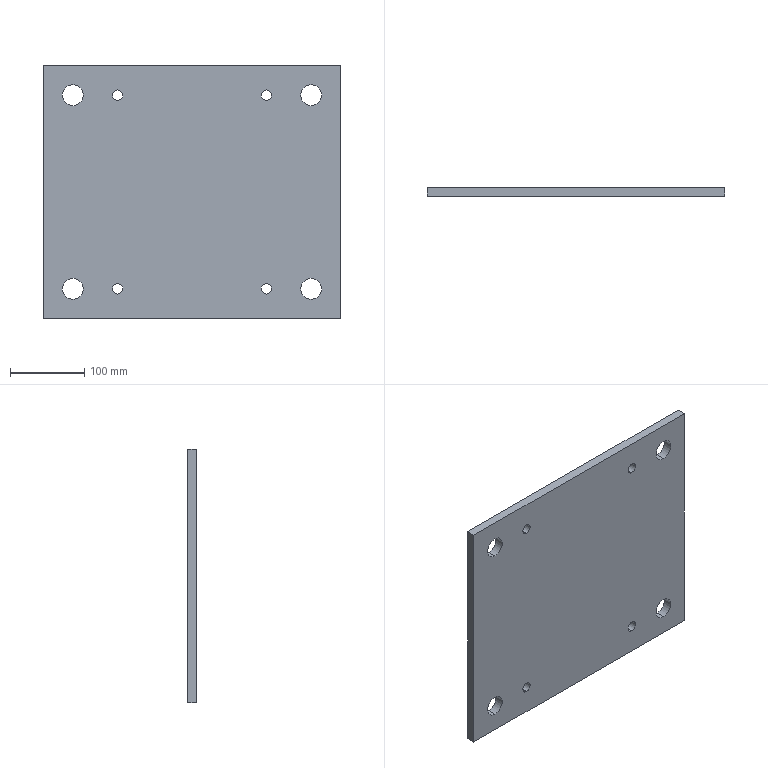Part | STEP file | Column base plate-Transfer kettle | 1 solid | 22 faces | box 400 x 12 x 340 mm | volume 1595055 mm3 | cylinder 16 | plane 6 | commonest cylinder face diameters 14 x8 28 x8